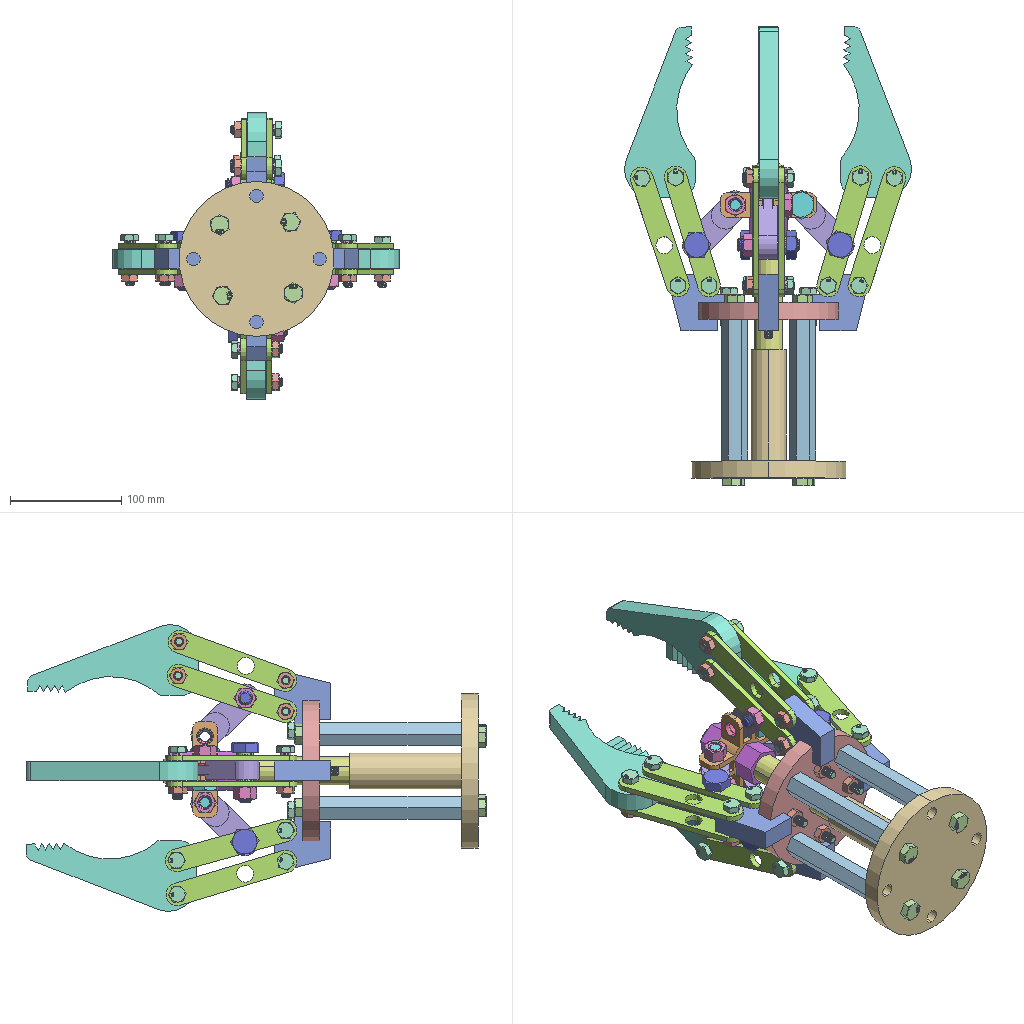Assembly | SolidWorks | 20 different items | 128 placed | box 258 x 413 x 257 mm
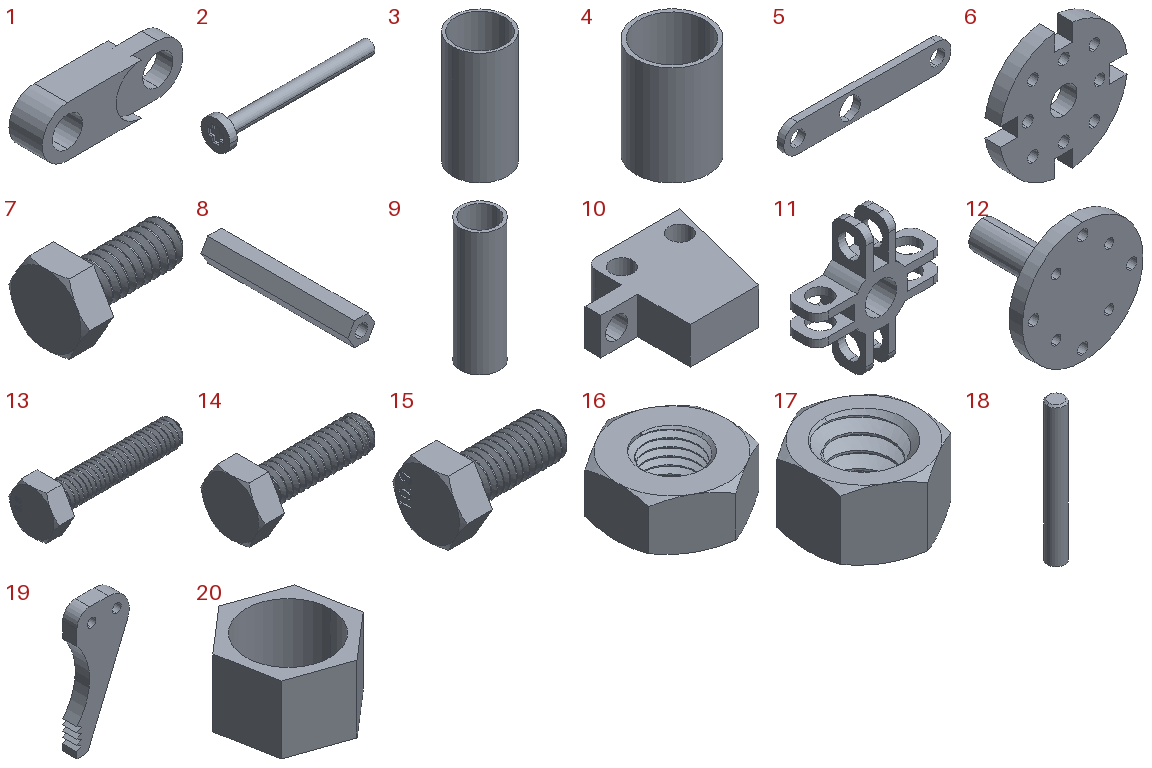Parts list (item | quantity | size | volume | features):
1 | x4 | 75.4 x 16.764 x 25.4 mm | 18082 mm3 | features ICE 3, Extrusion 1, Scale 1
2 | x1 | 133.35 x 25.4 x 25.4 mm | 16568 mm3 | features Fillet 1, ICE 1, Revolution 1
3 | x4 | 14.732 x 14.732 x 30.48 mm | 1019 mm3 | features Extrusion 1, Scale 1
4 | x5 | 14.732 x 14.732 x 20.32 mm | 679.556 mm3 | features Extrusion 1, Scale 1
5 | x16 | 121.92 x 5.08 x 20.32 mm | 10300 mm3 | features Extrusion 1, Scale 1
6 | x1 | 125.749 x 15.24 x 125.749 mm | 154760 mm3 | features ICE 2, CirPattern 1, Extrusion 1, Scale 1
7 | x4 | 39.211 x 25.663 x 22.225 mm | 6651 mm3 | features ICE 2, Chamfer 1, Extrusion 1, Helix 1, Revolution 1, Scale 1, SweepCut 1
8 | x4 | 23.464 x 127 x 20.32 mm | 34061 mm3 | features Extrusion 1, ICE 1, Scale 1
9 | x16 | 9.652 x 9.652 x 30.48 mm | 648.667 mm3 | features Extrusion 1, Scale 1
10 | x4 | 63.5 x 50.8 x 17.78 mm | 34011 mm3 | features Extrusion 1, Fillet 1, ICE 1, Scale 1
11 | x1 | 86.36 x 22.86 x 86.36 mm | 32385 mm3 | features ICE 4, CirPattern 1, Extrusion 1, Fillet 1, HoleWzd 1, Scale 1
12 | x1 | 139 x 115.24 x 139 mm | 246251 mm3 | features ICE 4, Cut 1, Extrusion 1, Scale 1
13 | x20 | 45.6 x 16.166 x 14 mm | 2539 mm3 | features ICE 3, Chamfer 1, Extrusion 1, Helix 1, Revolution 1, Scale 1, SweepCut 1
14 | x4 | 53.181 x 25.663 x 22.225 mm | 8007 mm3 | features ICE 2, Chamfer 1, Extrusion 1, Helix 1, Revolution 1, Scale 1, SweepCut 1
15 | x8 | 31 x 18.475 x 16 mm | 3064 mm3 | features ICE 3, Chamfer 1, Extrusion 1, Helix 1, Revolution 1, Scale 1, SweepCut 1
16 | x20 | 14 x 16.166 x 6.4 mm | 804.072 mm3 | features ICE 4, CombineBodies 1, Extrusion 1, Helix 1, MirrorPattern 1, Scale 1, SweepCut 1
17 | x8 | 17.78 x 20.531 x 11.113 mm | 1918 mm3 | features Extrusion 1, Helix 1, ICE 1, MirrorPattern 1, RevCut 1, Scale 1, Sweep 1
18 | x1 | 25.4 x 25.4 x 200 mm | 101101 mm3 | features Chamfer 1, Extrusion 1, Scale 1
19 | x4 | 63.5 x 17.272 x 152.4 mm | 90763 mm3 | features Fillet 3, ICE 2, Extrusion 1, Scale 1
20 | x2 | 33.572 x 34.936 x 20.32 mm | 6393 mm3 | features Extrusion 1, Scale 1
Mates (type | each side: item.copy, entity, surface, feature):
Concentric | 6.1 face cylinder Cut-Extrude2 | 10.1 face cylinder Cut-Extrude1
Coincident | 6.1 face plane Boss-Extrude1 | 10.1 face plane Boss-Extrude1
Concentric | 6.1 face cylinder Cut-Extrude2 | 10.2 face cylinder Cut-Extrude1
Coincident | 6.1 face plane Cut-Extrude1 | 10.2 face plane Boss-Extrude1
Coincident | 6.1 face plane Boss-Extrude1 | 10.2 face plane Boss-Extrude1
Concentric | 6.1 face cylinder Cut-Extrude2 | 10.3 face cylinder Cut-Extrude1
Coincident | 6.1 face plane CirPattern1 | 10.3 face plane Boss-Extrude1
Coincident | 6.1 face plane Boss-Extrude1 | 10.3 face plane Boss-Extrude1
Concentric | 6.1 face cylinder Cut-Extrude2 | 10.4 face cylinder Cut-Extrude1
Coincident | 6.1 face plane CirPattern1 | 10.4 face plane Boss-Extrude1
Coincident | 6.1 face plane Boss-Extrude1 | 10.4 face plane Boss-Extrude1
Concentric | 10.4 face cylinder Boss-Extrude1 | 5.1 face cylinder Boss-Extrude1
DistanceDim | 5.1 face plane Boss-Extrude1 | 10.4 face plane Boss-Extrude1
Concentric | 10.4 face cylinder Boss-Extrude1 | 5.2 face cylinder Boss-Extrude1
DistanceDim | 5.2 face plane Boss-Extrude1 | 10.4 face plane Boss-Extrude1
Concentric | 10.4 face cylinder Boss-Extrude1 | 9.1 face cylinder Boss-Extrude1
Coincident | 5.2 face plane Boss-Extrude1 | 9.1 face plane Boss-Extrude1
Coincident | 5.1 face plane Boss-Extrude1 | 5.2 face plane Boss-Extrude1
Concentric | 10.4 face cylinder Boss-Extrude1 | 5.3 face cylinder Boss-Extrude1
DistanceDim | 10.4 face plane Boss-Extrude1 | 5.3 face plane Boss-Extrude1
Concentric | 10.4 face cylinder Boss-Extrude1 | 5.4 face cylinder Boss-Extrude1
DistanceDim | 5.4 face plane Boss-Extrude1 | 10.4 face plane Boss-Extrude1
Coincident | 5.3 face plane Boss-Extrude1 | 5.4 face plane Boss-Extrude1
Concentric | 10.4 edge | 9.2 face cylinder Boss-Extrude1
Coincident | 5.3 face plane Boss-Extrude1 | 9.2 face plane Boss-Extrude1
Concentric | 10.1 face cylinder Boss-Extrude1 | 5.5 face cylinder Boss-Extrude1
DistanceDim | 5.5 face plane Boss-Extrude1 | 10.1 face plane Boss-Extrude1
Concentric | 10.1 face cylinder Boss-Extrude1 | 5.6 face cylinder Boss-Extrude1
DistanceDim | 10.1 face plane Boss-Extrude1 | 5.6 face plane Boss-Extrude1
Coincident | 5.5 face plane Boss-Extrude1 | 5.6 face plane Boss-Extrude1
Coincident | 6.1 face plane CirPattern1 | 10.1 face plane Boss-Extrude1
Concentric | 5.2 face cylinder Boss-Extrude1 | 19.1 face cylinder Cut-Extrude1
Concentric | 5.3 face cylinder Boss-Extrude1 | 19.1 face cylinder Cut-Extrude1
DistanceDim | 19.1 face plane Boss-Extrude1 | 5.3 face plane Boss-Extrude1
Concentric | 19.1 face cylinder Cut-Extrude1 | 9.3 face cylinder Boss-Extrude1
Coincident | 5.3 face plane Boss-Extrude1 | 9.3 face plane Boss-Extrude1
Concentric | 5.2 face cylinder Boss-Extrude1 | 9.4 face cylinder Boss-Extrude1
Coincident | 5.2 face plane Boss-Extrude1 | 9.4 face plane Boss-Extrude1
Concentric | 10.1 face cylinder Boss-Extrude1 | 5.7 face cylinder Boss-Extrude1
DistanceDim | 10.1 face plane Boss-Extrude1 | 5.7 face plane Boss-Extrude1
Concentric | 10.1 face cylinder Boss-Extrude1 | 5.8 face cylinder Boss-Extrude1
DistanceDim | 5.8 face plane Boss-Extrude1 | 10.1 face plane Boss-Extrude1
Coincident | 5.7 face plane Boss-Extrude1 | 5.8 face plane Boss-Extrude1
Concentric | 5.7 face cylinder Boss-Extrude1 | 19.2 face cylinder Cut-Extrude1
Concentric | 5.6 face cylinder Boss-Extrude1 | 19.2 face cylinder Cut-Extrude1
DistanceDim | 19.2 face plane Boss-Extrude1 | 5.6 face plane Boss-Extrude1
Concentric | 10.1 face cylinder Boss-Extrude1 | 9.5 face cylinder Boss-Extrude1
Coincident | 5.6 face plane Boss-Extrude1 | 9.5 face plane Boss-Extrude1
Concentric | 10.1 face cylinder Boss-Extrude1 | 9.6 face cylinder Boss-Extrude1
Coincident | 5.7 face plane Boss-Extrude1 | 9.6 face plane Boss-Extrude1
Concentric | 19.2 face cylinder Cut-Extrude1 | 9.7 face cylinder Boss-Extrude1
Coincident | 5.6 face plane Boss-Extrude1 | 9.7 face plane Boss-Extrude1
Concentric | 19.2 face cylinder Cut-Extrude1 | 9.8 face cylinder Boss-Extrude1
Coincident | 5.7 face plane Boss-Extrude1 | 9.8 face plane Boss-Extrude1
Concentric | 5.6 face cylinder Boss-Extrude1 | 1.1 face cylinder Boss-Extrude1
DistanceDim | 5.5 face plane Boss-Extrude1 | 1.1 face plane Boss-Extrude1
Coincident | 11.1 edge | 1.1 face cylinder Boss-Extrude1
DistanceDim | 11.1 face plane CirPattern1 | 1.1 face plane Cut-Extrude3
Concentric | 5.2 face cylinder Boss-Extrude1 | 1.2 face cylinder Boss-Extrude1
Concentric | 11.1 face cylinder Cut-Extrude7 | 1.2 face cylinder Boss-Extrude1
DistanceDim | 5.1 face plane Boss-Extrude1 | 1.2 face plane Boss-Extrude1
Parallel | 6.1 face plane Boss-Extrude1 | 11.1 face plane Boss-Extrude1
Concentric | 10.2 face cylinder Boss-Extrude1 | 5.9 face cylinder Boss-Extrude1
DistanceDim | 5.9 face plane Boss-Extrude1 | 10.2 face plane Boss-Extrude1
Concentric | 10.2 face cylinder Boss-Extrude1 | 5.10 face cylinder Boss-Extrude1
DistanceDim | 5.10 face plane Boss-Extrude1 | 10.2 face plane Boss-Extrude1
Coincident | 5.9 face plane Boss-Extrude1 | 5.10 face plane Boss-Extrude1
Concentric | 10.2 face cylinder Boss-Extrude1 | 5.11 face cylinder Boss-Extrude1
DistanceDim | 5.11 face plane Boss-Extrude1 | 10.2 face plane Boss-Extrude1
Concentric | 5.10 face cylinder Boss-Extrude1 | 19.3 face cylinder Cut-Extrude1
Concentric | 10.2 face cylinder Boss-Extrude1 | 5.12 face cylinder Boss-Extrude1
DistanceDim | 5.12 face plane Boss-Extrude1 | 10.2 face plane Boss-Extrude1
Coincident | 19.3 face cylinder Cut-Extrude1 | 5.12 edge
Concentric | 5.11 edge | 19.3 face cylinder Cut-Extrude1
DistanceDim | 19.3 face plane Boss-Extrude1 | 5.10 face plane Boss-Extrude1
Concentric | 5.10 face cylinder Boss-Extrude1 | 1.3 face cylinder Boss-Extrude1
DistanceDim | 1.3 face plane Boss-Extrude1 | 5.9 face plane Boss-Extrude1
Concentric | 11.1 face cylinder Cut-Extrude6 | 1.3 face cylinder Boss-Extrude1
Concentric | 19.3 face cylinder Cut-Extrude1 | 9.9 face cylinder Boss-Extrude1
Coincident | 5.10 face plane Boss-Extrude1 | 9.9 face plane Boss-Extrude1
Concentric | 5.12 face cylinder Boss-Extrude1 | 9.10 face cylinder Boss-Extrude1
Coincident | 5.12 face plane Boss-Extrude1 | 9.10 face plane Boss-Extrude1
Concentric | 10.2 face cylinder Boss-Extrude1 | 9.11 face cylinder Boss-Extrude1
Coincident | 5.10 face plane Boss-Extrude1 | 9.11 face plane Boss-Extrude1
Concentric | 10.2 face cylinder Boss-Extrude1 | 9.12 face cylinder Boss-Extrude1
Coincident | 5.12 face plane Boss-Extrude1 | 9.12 face plane Boss-Extrude1
DistanceDim | 1.3 face plane Cut-Extrude3 | 11.1 face plane CirPattern1
Concentric | 10.3 face cylinder Boss-Extrude1 | 5.13 face cylinder Boss-Extrude1
DistanceDim | 5.13 face plane Boss-Extrude1 | 10.3 face plane Boss-Extrude1
Concentric | 10.3 face cylinder Boss-Extrude1 | 5.14 face cylinder Boss-Extrude1
DistanceDim | 5.14 face plane Boss-Extrude1 | 10.3 face plane Boss-Extrude1
Coincident | 5.13 face plane Boss-Extrude1 | 5.14 face plane Boss-Extrude1
Concentric | 10.3 face cylinder Boss-Extrude1 | 5.15 edge
DistanceDim | 5.15 face plane Boss-Extrude1 | 10.3 face plane Boss-Extrude1
Concentric | 10.3 face cylinder Boss-Extrude1 | 5.16 face cylinder Boss-Extrude1
DistanceDim | 10.3 face plane Boss-Extrude1 | 5.16 face plane Boss-Extrude1
Coincident | 5.15 face plane Boss-Extrude1 | 5.16 face plane Boss-Extrude1
Concentric | 5.13 face cylinder Boss-Extrude1 | 1.4 face cylinder Boss-Extrude1
DistanceDim | 1.4 face plane Boss-Extrude1 | 5.13 face plane Boss-Extrude1
Concentric | 11.1 face cylinder Cut-Extrude6 | 1.4 face cylinder Boss-Extrude1
Concentric | 5.13 face cylinder Boss-Extrude1 | 19.4 face cylinder Cut-Extrude1
Concentric | 5.16 face cylinder Boss-Extrude1 | 19.4 face cylinder Cut-Extrude1
DistanceDim | 19.4 face plane Boss-Extrude1 | 5.16 face plane Boss-Extrude1
Concentric | 19.4 face cylinder Cut-Extrude1 | 9.13 face cylinder Boss-Extrude1
Coincident | 5.13 face plane Boss-Extrude1 | 9.13 face plane Boss-Extrude1
Concentric | 19.4 face cylinder Cut-Extrude1 | 9.14 face cylinder Boss-Extrude1
Coincident | 5.16 face plane Boss-Extrude1 | 9.14 face plane Boss-Extrude1
Concentric | 1.2 face cylinder Boss-Extrude1 | 3.1 face cylinder Boss-Extrude1
Coincident | 5.2 face plane Boss-Extrude1 | 3.1 face plane Boss-Extrude1
Concentric | 1.1 face cylinder Boss-Extrude1 | 3.2 face cylinder Boss-Extrude1
Coincident | 5.6 face plane Boss-Extrude1 | 3.2 face plane Boss-Extrude1
Concentric | 1.2 face cylinder Boss-Extrude1 | 4.1 face cylinder Boss-Extrude1
Coincident | 11.1 face plane Boss-Extrude1 | 4.1 face plane Boss-Extrude1
Concentric | 1.1 face cylinder Boss-Extrude1 | 4.2 face cylinder Boss-Extrude1
Coincident | 11.1 face plane Boss-Extrude1 | 4.2 face plane Boss-Extrude1
Concentric | 1.3 face cylinder Boss-Extrude1 | 4.3 face cylinder Boss-Extrude1
Coincident | 11.1 face plane Boss-Extrude1 | 4.3 face plane Boss-Extrude1
Concentric | 1.4 face cylinder Boss-Extrude1 | 4.4 face cylinder Boss-Extrude1
Coincident | 5.13 face plane Boss-Extrude1 | 4.4 face plane Boss-Extrude1
Concentric | 6.1 face cylinder Boss-Extrude1 | 8.1 face cylinder Cut-Extrude1
Coincident | 6.1 face plane Boss-Extrude1 | 8.1 face plane Boss-Extrude1
Concentric | 6.1 face cylinder Boss-Extrude1 | 8.2 face cylinder Cut-Extrude1
Coincident | 6.1 face plane Boss-Extrude1 | 8.2 face plane Boss-Extrude1
Concentric | 6.1 face cylinder Boss-Extrude1 | 8.3 face cylinder Cut-Extrude1
Coincident | 6.1 face plane Boss-Extrude1 | 8.3 face plane Boss-Extrude1
Concentric | 6.1 face cylinder Boss-Extrude1 | 8.4 face cylinder Cut-Extrude1
Coincident | 6.1 face plane Boss-Extrude1 | 8.4 face plane Boss-Extrude1
Concentric | 18.1 face cylinder Boss-Extrude1 | 20.1 face cylinder Boss-Extrude1
DistanceDim | 20.1 face plane Boss-Extrude1 | 18.1 face plane Boss-Extrude1
Coincident | 11.1 face plane Boss-Extrude1 | 20.1 face plane Boss-Extrude1
Concentric | 18.1 face cylinder Boss-Extrude1 | 20.2 face cylinder Boss-Extrude1
Coincident | 11.1 face plane Boss-Extrude1 | 20.2 face plane Boss-Extrude1
Concentric | 9.5 face cylinder Boss-Extrude1 | 13.1 edge
Coincident | 9.5 face plane Boss-Extrude1 | 13.1 face plane Boss-Extrude2
Concentric | 13.1 edge | 16.1 edge
Coincident | 5.6 face plane Boss-Extrude1 | 16.1 face plane Extrude1
Concentric | 9.6 face cylinder Boss-Extrude1 | 13.2 face cone Chamfer1
Coincident | 9.6 face plane Boss-Extrude1 | 13.2 face plane Boss-Extrude2
Concentric | 10.3 face cylinder Boss-Extrude1 | 9.15 face cylinder Boss-Extrude1
Coincident | 5.13 face plane Boss-Extrude1 | 9.15 face plane Boss-Extrude1
Concentric | 5.16 face cylinder Boss-Extrude1 | 9.16 face cylinder Boss-Extrude1
Coincident | 5.16 face plane Boss-Extrude1 | 9.16 face plane Boss-Extrude1
Concentric | 5.14 face cylinder Boss-Extrude1 | 3.3 face cylinder Boss-Extrude1
Coincident | 5.13 face plane Boss-Extrude1 | 3.3 face plane Boss-Extrude1
Concentric | 1.3 face cylinder Boss-Extrude1 | 3.4 face cylinder Boss-Extrude1
Coincident | 5.10 face plane Boss-Extrude1 | 3.4 face plane Boss-Extrude1
Concentric | 9.11 face cylinder Boss-Extrude1 | 13.3 face cone Chamfer1
Coincident | 9.11 face plane Boss-Extrude1 | 13.3 face plane Boss-Extrude2
Concentric | 9.12 face cylinder Boss-Extrude1 | 13.4 face cone Chamfer1
Coincident | 9.12 face plane Boss-Extrude1 | 13.4 face plane Boss-Extrude2
Concentric | 9.1 face cylinder Boss-Extrude1 | 13.5 face cone Chamfer1
Coincident | 9.1 face plane Boss-Extrude1 | 13.5 face plane Boss-Extrude2
Concentric | 9.2 face cylinder Boss-Extrude1 | 13.6 face cone Chamfer1
Coincident | 9.2 face plane Boss-Extrude1 | 13.6 face plane Boss-Extrude2
Concentric | 13.7 face cone Chamfer1 | 9.16 face cylinder Boss-Extrude1
Concentric | 13.8 face cone Chamfer1 | 9.15 face cylinder Boss-Extrude1
Coincident | 13.8 face plane Boss-Extrude2 | 9.15 face plane Boss-Extrude1
Coincident | 13.7 face plane Boss-Extrude2 | 9.16 face plane Boss-Extrude1
Concentric | 13.7 edge | 16.2 edge
Coincident | 5.16 face plane Boss-Extrude1 | 16.2 face plane Extrude1
Concentric | 13.8 face cone Chamfer1 | 16.3 edge
Coincident | 5.13 face plane Boss-Extrude1 | 16.3 face plane Extrude1
Concentric | 13.6 face cone Chamfer1 | 16.4 edge
Coincident | 5.3 face plane Boss-Extrude1 | 16.4 face plane Extrude1
Concentric | 13.5 face cone Chamfer1 | 16.5 face cone Cut-Extrude3
Coincident | 5.2 face plane Boss-Extrude1 | 16.5 face plane Extrude1
Concentric | 13.3 face cone Chamfer1 | 16.6 edge
Coincident | 5.10 face plane Boss-Extrude1 | 16.6 face plane Extrude1
Concentric | 13.4 face cone Chamfer1 | 16.7 edge
Coincident | 5.12 face plane Boss-Extrude1 | 16.7 face plane Extrude1
Concentric | 13.2 face cone Chamfer1 | 16.8 edge
Coincident | 5.7 face plane Boss-Extrude1 | 16.8 face plane Extrude1
Concentric | 6.1 face cylinder Boss-Extrude1 | 15.1 face cone Chamfer1
Coincident | 6.1 face plane Boss-Extrude1 | 15.1 face plane Boss-Extrude2
Concentric | 6.1 face cylinder Boss-Extrude1 | 15.2 face cone Chamfer1
Coincident | 6.1 face plane Boss-Extrude1 | 15.2 face plane Boss-Extrude2
Concentric | 6.1 face cylinder Boss-Extrude1 | 15.3 face cone Chamfer1
Coincident | 6.1 face plane Boss-Extrude1 | 15.3 face plane Boss-Extrude2
Concentric | 6.1 face cylinder Boss-Extrude1 | 15.4 face cone Chamfer1
Coincident | 6.1 face plane Boss-Extrude1 | 15.4 face plane Boss-Extrude2
Concentric | 9.10 face cylinder Boss-Extrude1 | 13.9 face cone Chamfer1
Concentric | 9.9 face cylinder Boss-Extrude1 | 13.10 face cone Chamfer1
Coincident | 9.9 face plane Boss-Extrude1 | 13.10 face plane Boss-Extrude2
Coincident | 9.10 face plane Boss-Extrude1 | 13.9 face plane Boss-Extrude2
Concentric | 13.9 face cone Chamfer1 | 16.9 face cone Cut-Extrude3
Coincident | 5.12 face plane Boss-Extrude1 | 16.9 face plane Extrude1
Concentric | 13.10 face cone Chamfer1 | 16.10 face cone Cut-Extrude3
Coincident | 5.10 face plane Boss-Extrude1 | 16.10 face plane Extrude1
Concentric | 9.14 face cylinder Boss-Extrude1 | 13.11 face cone Chamfer1
Concentric | 9.13 face cylinder Boss-Extrude1 | 13.12 face cone Chamfer1
Coincident | 9.13 face plane Boss-Extrude1 | 13.12 face plane Boss-Extrude2
Coincident | 9.14 face plane Boss-Extrude1 | 13.11 face plane Boss-Extrude2
Concentric | 13.11 face cone Chamfer1 | 16.11 face cone Cut-Extrude2
Coincident | 5.16 face plane Boss-Extrude1 | 16.11 face plane Extrude1
Concentric | 13.12 face cone Chamfer1 | 16.12 face cone Cut-Extrude2
Coincident | 5.13 face plane Boss-Extrude1 | 16.12 face plane Extrude1
Concentric | 9.8 face cylinder Boss-Extrude1 | 13.13 face cone Chamfer1
Concentric | 9.7 face cylinder Boss-Extrude1 | 13.14 face cone Chamfer1
Coincident | 5.8 face plane Boss-Extrude1 | 13.13 face plane Boss-Extrude2
Coincident | 5.5 face plane Boss-Extrude1 | 13.14 face plane Boss-Extrude2
Concentric | 13.14 face cone Chamfer1 | 16.13 face cone Cut-Extrude2
Coincident | 5.6 face plane Boss-Extrude1 | 16.13 face plane Extrude1
Concentric | 13.13 face cone Chamfer1 | 16.14 face cone Cut-Extrude3
Coincident | 5.7 face plane Boss-Extrude1 | 16.14 face plane Extrude1
Concentric | 9.4 face cylinder Boss-Extrude1 | 13.15 face cone Chamfer1
Concentric | 9.3 face cylinder Boss-Extrude1 | 13.16 face cone Chamfer1
Coincident | 9.3 face plane Boss-Extrude1 | 13.16 face plane Boss-Extrude2
Coincident | 9.4 face plane Boss-Extrude1 | 13.15 face plane Boss-Extrude2
Concentric | 13.16 face cone Chamfer1 | 16.15 face cone Cut-Extrude2
Coincident | 5.3 face plane Boss-Extrude1 | 16.15 face plane Extrude1
Concentric | 13.15 face cone Chamfer1 | 16.16 face cone Cut-Extrude3
Coincident | 5.2 face plane Boss-Extrude1 | 16.16 face plane Extrude1
Concentric | 3.2 face cylinder Boss-Extrude1 | 14.1 face cone Chamfer1
Coincident | 3.2 face plane Boss-Extrude1 | 14.1 face plane Boss-Extrude4
Concentric | 3.3 face cylinder Boss-Extrude1 | 14.2 face cone Chamfer1
Concentric | 3.4 face cylinder Boss-Extrude1 | 14.3 face cone Chamfer1
Coincident | 3.4 face plane Boss-Extrude1 | 14.3 face plane Boss-Extrude4
Coincident | 3.3 face plane Boss-Extrude1 | 14.2 face plane Boss-Extrude4
Concentric | 14.4 face cone Chamfer1 | 17.1 face cone Mirror1
Coincident | 5.2 face plane Boss-Extrude1 | 17.1 face plane Extrude1
Concentric | 14.2 face cone Chamfer1 | 17.2 face cone Cut-Revolve1
Coincident | 5.13 face plane Boss-Extrude1 | 17.2 select_type:24
Concentric | 14.1 face cone Chamfer1 | 17.3 face cone Cut-Revolve1
Coincident | 5.6 face plane Boss-Extrude1 | 17.3 face plane Extrude1
Concentric | 14.3 face cone Chamfer1 | 17.4 face cone Cut-Revolve1
Coincident | 5.10 face plane Boss-Extrude1 | 17.4 face plane Extrude1
Concentric | 4.2 face cylinder Boss-Extrude1 | 7.1 face cone Chamfer1
Coincident | 11.1 face plane Boss-Extrude1 | 7.1 face plane Boss-Extrude4
Concentric | 11.1 face cylinder Cut-Extrude6 | 4.5 face cylinder Boss-Extrude1
Coincident | 11.1 face plane Boss-Extrude1 | 4.5 face plane Boss-Extrude1
Concentric | 7.2 face cone Chamfer1 | 4.5 face cylinder Boss-Extrude1
Coincident | 7.2 face plane Boss-Extrude4 | 4.5 face plane Boss-Extrude1
Concentric | 17.5 face cone Cut-Revolve1 | 7.2 face cone Chamfer1
Coincident | 11.1 face plane Boss-Extrude1 | 17.5 face plane Extrude1
Concentric | 4.1 face cylinder Boss-Extrude1 | 7.3 face cone Chamfer1
Coincident | 11.1 face plane Boss-Extrude1 | 7.3 face plane Boss-Extrude4
Concentric | 7.3 face cone Chamfer1 | 17.6 face cone Mirror1
Coincident | 11.1 face plane Boss-Extrude1 | 17.6 face plane Extrude1
Concentric | 4.3 face cylinder Boss-Extrude1 | 7.4 face cone Chamfer1
Coincident | 11.1 face plane Boss-Extrude1 | 7.4 face plane Boss-Extrude4
Concentric | 17.7 select_type:24 | 7.4 face cone Chamfer1
Coincident | 11.1 face plane Boss-Extrude1 | 17.7 face plane Extrude1
Concentric | 7.1 face cone Chamfer1 | 17.8 face cone Mirror1
Coincident | 11.1 face plane Boss-Extrude1 | 17.8 face plane Extrude1
Coincident | 15.5 face plane Boss-Extrude2 | 12.1 face plane Boss-Extrude1
Coincident | 8.3 face plane Boss-Extrude1 | 12.1 face plane Boss-Extrude1
Concentric | 8.3 face cylinder Cut-Extrude1 | 12.1 face cylinder Boss-Extrude1
Concentric | 8.4 face cylinder Cut-Extrude1 | 12.1 face cylinder Boss-Extrude1
Concentric | 15.5 edge | 12.1 face cylinder Boss-Extrude1
Concentric | 18.1 face cylinder Boss-Extrude1 | 12.1 face cylinder Boss-Extrude2
Concentric | 3.1 face cylinder Boss-Extrude1 | 14.4 edge
Coincident | 3.1 face plane Boss-Extrude1 | 14.4 face plane Boss-Extrude4
Concentric | 13.17 edge | 16.17 edge
Concentric | 10.1 face cylinder Cut-Extrude1 | 13.17 edge
Coincident | 10.1 face plane Boss-Extrude1 | 13.17 face plane Boss-Extrude2
Coincident | 6.1 face plane Boss-Extrude1 | 16.17 face plane Extrude1